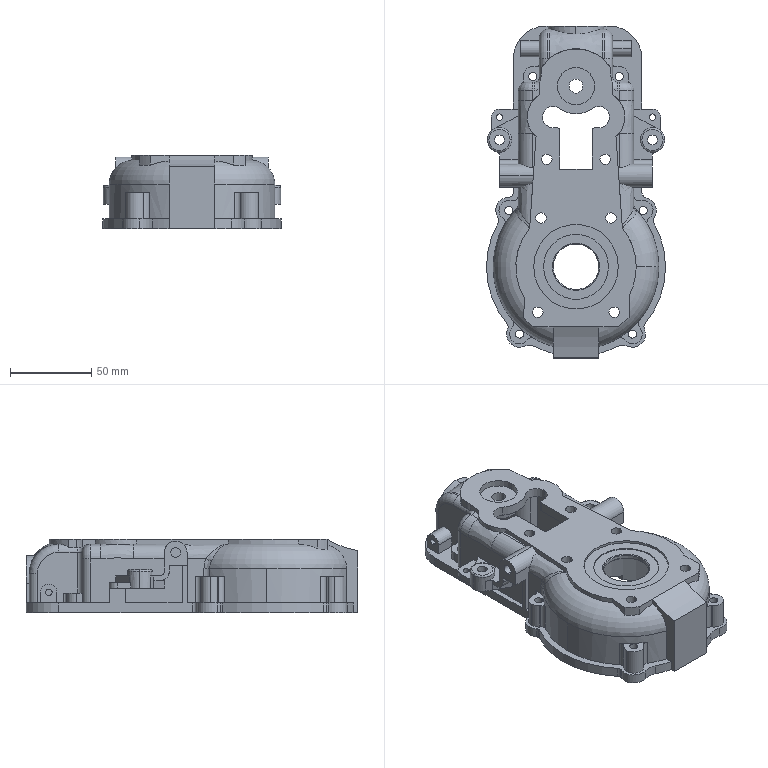Part | SolidWorks | features BaseBody 1 | 1 solid | 361 faces | box 110 x 204 x 45 mm | volume 158964 mm3 | cylinder 182 | plane 150 | torus 16 | spline 9 | cone 4 | commonest cylinder face diameters 6 x30 10 x15 4 x12 5 x12 6.5 x12 14 x12